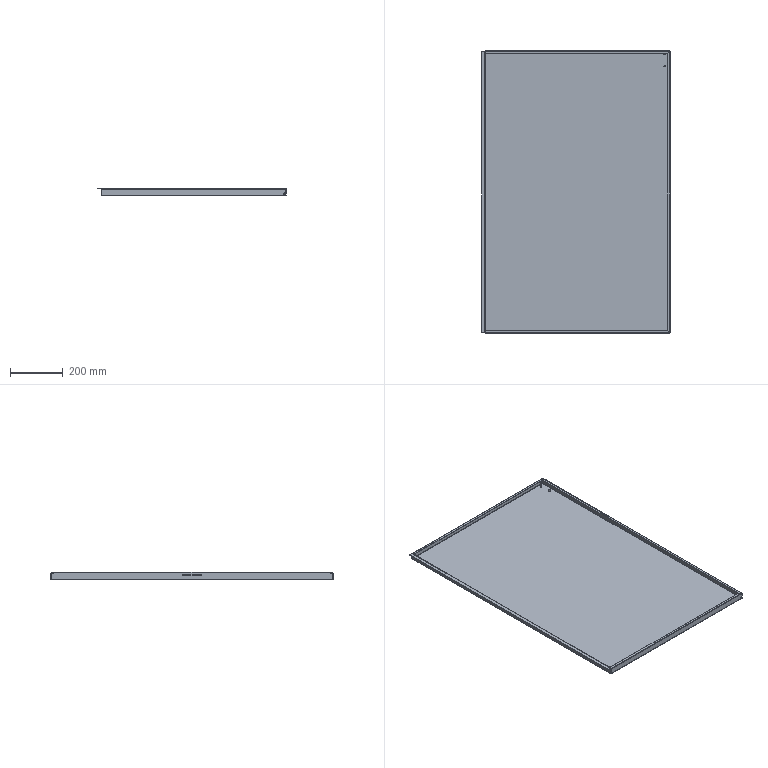Part | SolidWorks | features EdgeFlange 3, ICE 3, Fillet 1, FlatPattern 1, LPattern 1, SMBaseFlange 1, SheetMetal 1 | 1 solid | 86 faces | box 713.5 x 1066 x 27.237 mm | volume 1292655 mm3 | plane 48 | cylinder 26 | spline 12 | commonest cylinder face diameters 1.473 x8 4.473 x8 5 x4 6.3 x4 10 x2